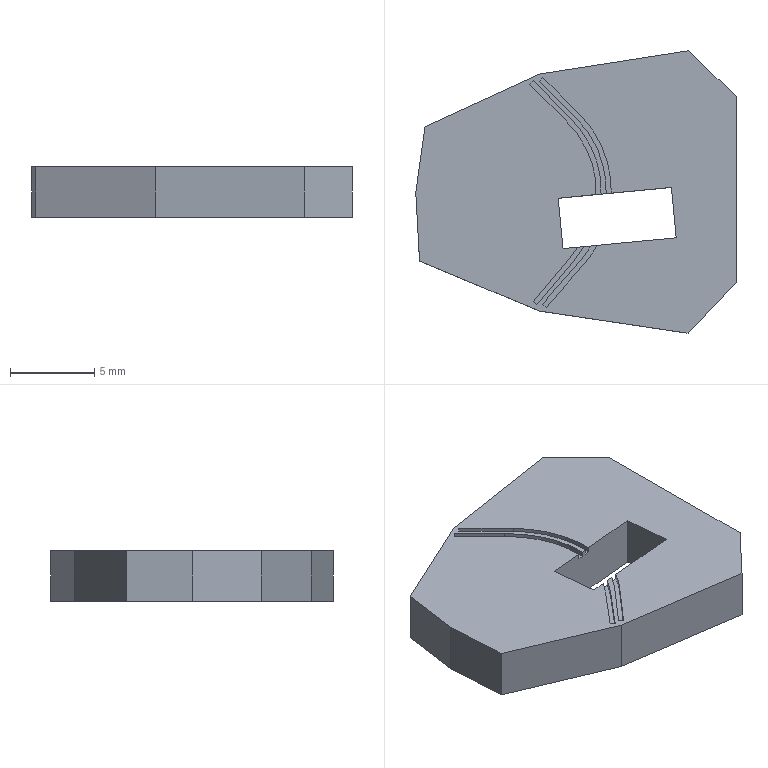Part | SolidWorks | features BaseBody 1 | 1 solid | 39 faces | box 19 x 16.741 x 3 mm | volume 696.97 mm3 | spline 20 | plane 19